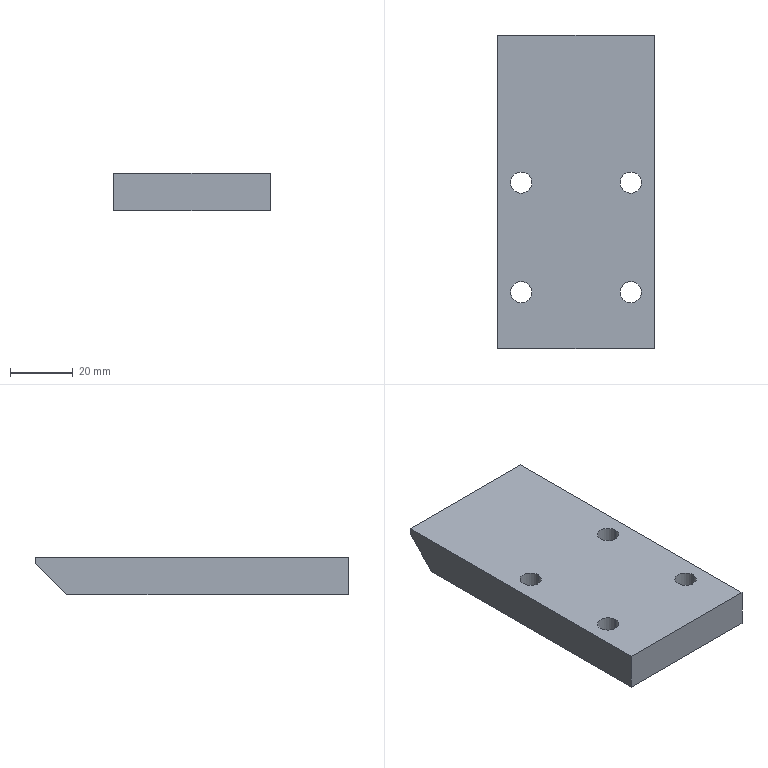Part | STEP file | BCC3 H11_2B1 | 1 solid | 15 faces | box 50 x 100 x 12 mm | volume 55757 mm3 | cylinder 8 | plane 7 | commonest cylinder face diameters 6.8 x8
STEP:
#1=CARTESIAN_POINT('',(0.,0.,0.));
#2=DIRECTION('',(0.,0.,1.));
#3=DIRECTION('',(1.,0.,0.));
#4=AXIS2_PLACEMENT_3D('',#1,#2,#3);
#5=CARTESIAN_POINT('',(-14.1,3.,0.));
#6=VERTEX_POINT('',#5);
#7=CARTESIAN_POINT('',(-14.1,3.,12.));
#8=VERTEX_POINT('',#7);
#9=CARTESIAN_POINT('',(-14.1,3.,12.));
#10=DIRECTION('',(0.,0.,1.));
#11=VECTOR('',#10,1.);
#12=LINE('',#9,#11);
#13=CARTESIAN_POINT('',(-17.5,3.,12.));
#14=DIRECTION('',(0.,0.,1.));
#15=DIRECTION('',(1.,0.,0.));
#16=AXIS2_PLACEMENT_3D('',#13,#14,#15);
#17=CYLINDRICAL_SURFACE('',#16,3.4);
#18=CARTESIAN_POINT('',(6.283,0.));
#19=DIRECTION('',(0.,1.));
#20=VECTOR('',#19,1.);
#21=LINE('',#18,#20);
#22=(GEOMETRIC_REPRESENTATION_CONTEXT(2)PARAMETRIC_REPRESENTATION_CONTEXT()REPRESENTATION_CONTEXT('',''));
#23=DEFINITIONAL_REPRESENTATION('',(#21),#22);
#24=PCURVE('',#17,#23);
#25=CARTESIAN_POINT('',(-17.5,3.,12.));
#26=DIRECTION('',(0.,0.,1.));
#27=DIRECTION('',(1.,0.,0.));
#28=AXIS2_PLACEMENT_3D('',#25,#26,#27);
#29=CYLINDRICAL_SURFACE('',#28,3.4);
#30=CARTESIAN_POINT('',(0.,0.));
#31=DIRECTION('',(0.,1.));
#32=VECTOR('',#31,1.);
#33=LINE('',#30,#32);
#34=(GEOMETRIC_REPRESENTATION_CONTEXT(2)PARAMETRIC_REPRESENTATION_CONTEXT()REPRESENTATION_CONTEXT('',''));
#35=DEFINITIONAL_REPRESENTATION('',(#33),#34);
#36=PCURVE('',#29,#35);
#37=SURFACE_CURVE('',#12,(#24,#36),.PCURVE_S1.);
#38=EDGE_CURVE('',#6,#8,#37,.T.);
#39=ORIENTED_EDGE('',*,*,#38,.T.);
#40=CARTESIAN_POINT('',(-20.9,3.,12.));
#41=VERTEX_POINT('',#40);
#42=CARTESIAN_POINT('',(-17.5,3.,12.));
#43=DIRECTION('',(0.,0.,1.));
#44=DIRECTION('',(1.,0.,0.));
#45=AXIS2_PLACEMENT_3D('',#42,#43,#44);
#46=CIRCLE('',#45,3.4);
#47=CARTESIAN_POINT('',(0.,0.));
#48=DIRECTION('',(1.,0.));
#49=VECTOR('',#48,1.);
#50=LINE('',#47,#49);
#51=(GEOMETRIC_REPRESENTATION_CONTEXT(2)PARAMETRIC_REPRESENTATION_CONTEXT()REPRESENTATION_CONTEXT('',''));
#52=DEFINITIONAL_REPRESENTATION('',(#50),#51);
#53=PCURVE('',#17,#52);
#54=CARTESIAN_POINT('',(0.,0.,12.));
#55=DIRECTION('',(0.,0.,1.));
#56=DIRECTION('',(1.,0.,0.));
#57=AXIS2_PLACEMENT_3D('',#54,#55,#56);
#58=PLANE('',#57);
#59=CARTESIAN_POINT('',(-17.5,3.));
#60=DIRECTION('',(1.,0.));
#61=AXIS2_PLACEMENT_2D('',#59,#60);
#62=CIRCLE('',#61,3.4);
#63=(GEOMETRIC_REPRESENTATION_CONTEXT(2)PARAMETRIC_REPRESENTATION_CONTEXT()REPRESENTATION_CONTEXT('',''));
#64=DEFINITIONAL_REPRESENTATION('',(#62),#63);
#65=PCURVE('',#58,#64);
#66=SURFACE_CURVE('',#46,(#53,#65),.PCURVE_S1.);
#67=EDGE_CURVE('',#41,#8,#66,.T.);
#68=ORIENTED_EDGE('',*,*,#67,.F.);
#69=CARTESIAN_POINT('',(-20.9,3.,0.));
#70=VERTEX_POINT('',#69);
#71=CARTESIAN_POINT('',(-20.9,3.,12.));
#72=DIRECTION('',(0.,0.,1.));
#73=VECTOR('',#72,1.);
#74=LINE('',#71,#73);
#75=CARTESIAN_POINT('',(3.142,0.));
#76=DIRECTION('',(0.,1.));
#77=VECTOR('',#76,1.);
#78=LINE('',#75,#77);
#79=(GEOMETRIC_REPRESENTATION_CONTEXT(2)PARAMETRIC_REPRESENTATION_CONTEXT()REPRESENTATION_CONTEXT('',''));
#80=DEFINITIONAL_REPRESENTATION('',(#78),#79);
#81=PCURVE('',#17,#80);
#82=CARTESIAN_POINT('',(3.142,0.));
#83=DIRECTION('',(0.,1.));
#84=VECTOR('',#83,1.);
#85=LINE('',#82,#84);
#86=(GEOMETRIC_REPRESENTATION_CONTEXT(2)PARAMETRIC_REPRESENTATION_CONTEXT()REPRESENTATION_CONTEXT('',''));
#87=DEFINITIONAL_REPRESENTATION('',(#85),#86);
#88=PCURVE('',#29,#87);
#89=SURFACE_CURVE('',#74,(#81,#88),.PCURVE_S1.);
#90=EDGE_CURVE('',#70,#41,#89,.T.);
#91=ORIENTED_EDGE('',*,*,#90,.F.);
#92=CARTESIAN_POINT('',(-17.5,3.,0.));
#93=DIRECTION('',(0.,0.,1.));
#94=DIRECTION('',(1.,0.,0.));
#95=AXIS2_PLACEMENT_3D('',#92,#93,#94);
#96=CIRCLE('',#95,3.4);
#97=CARTESIAN_POINT('',(0.,-12.));
#98=DIRECTION('',(1.,0.));
#99=VECTOR('',#98,1.);
#100=LINE('',#97,#99);
#101=(GEOMETRIC_REPRESENTATION_CONTEXT(2)PARAMETRIC_REPRESENTATION_CONTEXT()REPRESENTATION_CONTEXT('',''));
#102=DEFINITIONAL_REPRESENTATION('',(#100),#101);
#103=PCURVE('',#17,#102);
#104=CARTESIAN_POINT('',(0.,0.,0.));
#105=DIRECTION('',(0.,0.,1.));
#106=DIRECTION('',(1.,0.,0.));
#107=AXIS2_PLACEMENT_3D('',#104,#105,#106);
#108=PLANE('',#107);
#109=CARTESIAN_POINT('',(-17.5,3.));
#110=DIRECTION('',(1.,0.));
#111=AXIS2_PLACEMENT_2D('',#109,#110);
#112=CIRCLE('',#111,3.4);
#113=(GEOMETRIC_REPRESENTATION_CONTEXT(2)PARAMETRIC_REPRESENTATION_CONTEXT()REPRESENTATION_CONTEXT('',''));
#114=DEFINITIONAL_REPRESENTATION('',(#112),#113);
#115=PCURVE('',#108,#114);
#116=SURFACE_CURVE('',#96,(#103,#115),.PCURVE_S1.);
#117=EDGE_CURVE('',#70,#6,#116,.T.);
#118=ORIENTED_EDGE('',*,*,#117,.T.);
#119=EDGE_LOOP('',(#39,#68,#91,#118));
#120=FACE_BOUND('',#119,.F.);
#121=ADVANCED_FACE('',(#120),#17,.F.);
#122=CARTESIAN_POINT('',(20.9,3.,0.));
#123=VERTEX_POINT('',#122);
#124=CARTESIAN_POINT('',(20.9,3.,12.));
#125=VERTEX_POINT('',#124);
#126=CARTESIAN_POINT('',(20.9,3.,12.));
#127=DIRECTION('',(0.,0.,1.));
#128=VECTOR('',#127,1.);
#129=LINE('',#126,#128);
#130=CARTESIAN_POINT('',(17.5,3.,12.));
#131=DIRECTION('',(0.,0.,1.));
#132=DIRECTION('',(1.,0.,0.));
#133=AXIS2_PLACEMENT_3D('',#130,#131,#132);
#134=CYLINDRICAL_SURFACE('',#133,3.4);
#135=CARTESIAN_POINT('',(6.283,0.));
#136=DIRECTION('',(0.,1.));
#137=VECTOR('',#136,1.);
#138=LINE('',#135,#137);
#139=(GEOMETRIC_REPRESENTATION_CONTEXT(2)PARAMETRIC_REPRESENTATION_CONTEXT()REPRESENTATION_CONTEXT('',''));
#140=DEFINITIONAL_REPRESENTATION('',(#138),#139);
#141=PCURVE('',#134,#140);
#142=CARTESIAN_POINT('',(17.5,3.,12.));
#143=DIRECTION('',(0.,0.,1.));
#144=DIRECTION('',(1.,0.,0.));
#145=AXIS2_PLACEMENT_3D('',#142,#143,#144);
#146=CYLINDRICAL_SURFACE('',#145,3.4);
#147=CARTESIAN_POINT('',(0.,0.));
#148=DIRECTION('',(0.,1.));
#149=VECTOR('',#148,1.);
#150=LINE('',#147,#149);
#151=(GEOMETRIC_REPRESENTATION_CONTEXT(2)PARAMETRIC_REPRESENTATION_CONTEXT()REPRESENTATION_CONTEXT('',''));
#152=DEFINITIONAL_REPRESENTATION('',(#150),#151);
#153=PCURVE('',#146,#152);
#154=SURFACE_CURVE('',#129,(#141,#153),.PCURVE_S1.);
#155=EDGE_CURVE('',#123,#125,#154,.T.);
#156=ORIENTED_EDGE('',*,*,#155,.T.);
#157=CARTESIAN_POINT('',(14.1,3.,12.));
#158=VERTEX_POINT('',#157);
#159=CARTESIAN_POINT('',(17.5,3.,12.));
#160=DIRECTION('',(0.,0.,1.));
#161=DIRECTION('',(1.,0.,0.));
#162=AXIS2_PLACEMENT_3D('',#159,#160,#161);
#163=CIRCLE('',#162,3.4);
#164=CARTESIAN_POINT('',(0.,0.));
#165=DIRECTION('',(1.,0.));
#166=VECTOR('',#165,1.);
#167=LINE('',#164,#166);
#168=(GEOMETRIC_REPRESENTATION_CONTEXT(2)PARAMETRIC_REPRESENTATION_CONTEXT()REPRESENTATION_CONTEXT('',''));
#169=DEFINITIONAL_REPRESENTATION('',(#167),#168);
#170=PCURVE('',#134,#169);
#171=CARTESIAN_POINT('',(17.5,3.));
#172=DIRECTION('',(1.,0.));
#173=AXIS2_PLACEMENT_2D('',#171,#172);
#174=CIRCLE('',#173,3.4);
#175=(GEOMETRIC_REPRESENTATION_CONTEXT(2)PARAMETRIC_REPRESENTATION_CONTEXT()REPRESENTATION_CONTEXT('',''));
#176=DEFINITIONAL_REPRESENTATION('',(#174),#175);
#177=PCURVE('',#58,#176);
#178=SURFACE_CURVE('',#163,(#170,#177),.PCURVE_S1.);
#179=EDGE_CURVE('',#158,#125,#178,.T.);
#180=ORIENTED_EDGE('',*,*,#179,.F.);
#181=CARTESIAN_POINT('',(14.1,3.,0.));
#182=VERTEX_POINT('',#181);
#183=CARTESIAN_POINT('',(14.1,3.,12.));
#184=DIRECTION('',(0.,0.,1.));
#185=VECTOR('',#184,1.);
#186=LINE('',#183,#185);
#187=CARTESIAN_POINT('',(3.142,0.));
#188=DIRECTION('',(0.,1.));
#189=VECTOR('',#188,1.);
#190=LINE('',#187,#189);
#191=(GEOMETRIC_REPRESENTATION_CONTEXT(2)PARAMETRIC_REPRESENTATION_CONTEXT()REPRESENTATION_CONTEXT('',''));
#192=DEFINITIONAL_REPRESENTATION('',(#190),#191);
#193=PCURVE('',#134,#192);
#194=CARTESIAN_POINT('',(3.142,0.));
#195=DIRECTION('',(0.,1.));
#196=VECTOR('',#195,1.);
#197=LINE('',#194,#196);
#198=(GEOMETRIC_REPRESENTATION_CONTEXT(2)PARAMETRIC_REPRESENTATION_CONTEXT()REPRESENTATION_CONTEXT('',''));
#199=DEFINITIONAL_REPRESENTATION('',(#197),#198);
#200=PCURVE('',#146,#199);
#201=SURFACE_CURVE('',#186,(#193,#200),.PCURVE_S1.);
#202=EDGE_CURVE('',#182,#158,#201,.T.);
#203=ORIENTED_EDGE('',*,*,#202,.F.);
#204=CARTESIAN_POINT('',(17.5,3.,0.));
#205=DIRECTION('',(0.,0.,1.));
#206=DIRECTION('',(1.,0.,0.));
#207=AXIS2_PLACEMENT_3D('',#204,#205,#206);
#208=CIRCLE('',#207,3.4);
#209=CARTESIAN_POINT('',(0.,-12.));
#210=DIRECTION('',(1.,0.));
#211=VECTOR('',#210,1.);
#212=LINE('',#209,#211);
#213=(GEOMETRIC_REPRESENTATION_CONTEXT(2)PARAMETRIC_REPRESENTATION_CONTEXT()REPRESENTATION_CONTEXT('',''));
#214=DEFINITIONAL_REPRESENTATION('',(#212),#213);
#215=PCURVE('',#134,#214);
#216=CARTESIAN_POINT('',(17.5,3.));
#217=DIRECTION('',(1.,0.));
#218=AXIS2_PLACEMENT_2D('',#216,#217);
#219=CIRCLE('',#218,3.4);
#220=(GEOMETRIC_REPRESENTATION_CONTEXT(2)PARAMETRIC_REPRESENTATION_CONTEXT()REPRESENTATION_CONTEXT('',''));
#221=DEFINITIONAL_REPRESENTATION('',(#219),#220);
#222=PCURVE('',#108,#221);
#223=SURFACE_CURVE('',#208,(#215,#222),.PCURVE_S1.);
#224=EDGE_CURVE('',#182,#123,#223,.T.);
#225=ORIENTED_EDGE('',*,*,#224,.T.);
#226=EDGE_LOOP('',(#156,#180,#203,#225));
#227=FACE_BOUND('',#226,.F.);
#228=ADVANCED_FACE('',(#227),#134,.F.);
#229=CARTESIAN_POINT('',(20.9,-32.,0.));
#230=VERTEX_POINT('',#229);
#231=CARTESIAN_POINT('',(20.9,-32.,12.));
#232=VERTEX_POINT('',#231);
#233=CARTESIAN_POINT('',(20.9,-32.,12.));
#234=DIRECTION('',(0.,0.,1.));
#235=VECTOR('',#234,1.);
#236=LINE('',#233,#235);
#237=CARTESIAN_POINT('',(17.5,-32.,12.));
#238=DIRECTION('',(0.,0.,1.));
#239=DIRECTION('',(1.,0.,0.));
#240=AXIS2_PLACEMENT_3D('',#237,#238,#239);
#241=CYLINDRICAL_SURFACE('',#240,3.4);
#242=CARTESIAN_POINT('',(6.283,0.));
#243=DIRECTION('',(0.,1.));
#244=VECTOR('',#243,1.);
#245=LINE('',#242,#244);
#246=(GEOMETRIC_REPRESENTATION_CONTEXT(2)PARAMETRIC_REPRESENTATION_CONTEXT()REPRESENTATION_CONTEXT('',''));
#247=DEFINITIONAL_REPRESENTATION('',(#245),#246);
#248=PCURVE('',#241,#247);
#249=CARTESIAN_POINT('',(17.5,-32.,12.));
#250=DIRECTION('',(0.,0.,1.));
#251=DIRECTION('',(1.,0.,0.));
#252=AXIS2_PLACEMENT_3D('',#249,#250,#251);
#253=CYLINDRICAL_SURFACE('',#252,3.4);
#254=CARTESIAN_POINT('',(0.,0.));
#255=DIRECTION('',(0.,1.));
#256=VECTOR('',#255,1.);
#257=LINE('',#254,#256);
#258=(GEOMETRIC_REPRESENTATION_CONTEXT(2)PARAMETRIC_REPRESENTATION_CONTEXT()REPRESENTATION_CONTEXT('',''));
#259=DEFINITIONAL_REPRESENTATION('',(#257),#258);
#260=PCURVE('',#253,#259);
#261=SURFACE_CURVE('',#236,(#248,#260),.PCURVE_S1.);
#262=EDGE_CURVE('',#230,#232,#261,.T.);
#263=ORIENTED_EDGE('',*,*,#262,.T.);
#264=CARTESIAN_POINT('',(14.1,-32.,12.));
#265=VERTEX_POINT('',#264);
#266=CARTESIAN_POINT('',(17.5,-32.,12.));
#267=DIRECTION('',(0.,0.,1.));
#268=DIRECTION('',(1.,0.,0.));
#269=AXIS2_PLACEMENT_3D('',#266,#267,#268);
#270=CIRCLE('',#269,3.4);
#271=CARTESIAN_POINT('',(0.,0.));
#272=DIRECTION('',(1.,0.));
#273=VECTOR('',#272,1.);
#274=LINE('',#271,#273);
#275=(GEOMETRIC_REPRESENTATION_CONTEXT(2)PARAMETRIC_REPRESENTATION_CONTEXT()REPRESENTATION_CONTEXT('',''));
#276=DEFINITIONAL_REPRESENTATION('',(#274),#275);
#277=PCURVE('',#241,#276);
#278=CARTESIAN_POINT('',(17.5,-32.));
#279=DIRECTION('',(1.,0.));
#280=AXIS2_PLACEMENT_2D('',#278,#279);
#281=CIRCLE('',#280,3.4);
#282=(GEOMETRIC_REPRESENTATION_CONTEXT(2)PARAMETRIC_REPRESENTATION_CONTEXT()REPRESENTATION_CONTEXT('',''));
#283=DEFINITIONAL_REPRESENTATION('',(#281),#282);
#284=PCURVE('',#58,#283);
#285=SURFACE_CURVE('',#270,(#277,#284),.PCURVE_S1.);
#286=EDGE_CURVE('',#265,#232,#285,.T.);
#287=ORIENTED_EDGE('',*,*,#286,.F.);
#288=CARTESIAN_POINT('',(14.1,-32.,0.));
#289=VERTEX_POINT('',#288);
#290=CARTESIAN_POINT('',(14.1,-32.,12.));
#291=DIRECTION('',(0.,0.,1.));
#292=VECTOR('',#291,1.);
#293=LINE('',#290,#292);
#294=CARTESIAN_POINT('',(3.142,0.));
#295=DIRECTION('',(0.,1.));
#296=VECTOR('',#295,1.);
#297=LINE('',#294,#296);
#298=(GEOMETRIC_REPRESENTATION_CONTEXT(2)PARAMETRIC_REPRESENTATION_CONTEXT()REPRESENTATION_CONTEXT('',''));
#299=DEFINITIONAL_REPRESENTATION('',(#297),#298);
#300=PCURVE('',#241,#299);
#301=CARTESIAN_POINT('',(3.142,0.));
#302=DIRECTION('',(0.,1.));
#303=VECTOR('',#302,1.);
#304=LINE('',#301,#303);
#305=(GEOMETRIC_REPRESENTATION_CONTEXT(2)PARAMETRIC_REPRESENTATION_CONTEXT()REPRESENTATION_CONTEXT('',''));
#306=DEFINITIONAL_REPRESENTATION('',(#304),#305);
#307=PCURVE('',#253,#306);
#308=SURFACE_CURVE('',#293,(#300,#307),.PCURVE_S1.);
#309=EDGE_CURVE('',#289,#265,#308,.T.);
#310=ORIENTED_EDGE('',*,*,#309,.F.);
#311=CARTESIAN_POINT('',(17.5,-32.,0.));
#312=DIRECTION('',(0.,0.,1.));
#313=DIRECTION('',(1.,0.,0.));
#314=AXIS2_PLACEMENT_3D('',#311,#312,#313);
#315=CIRCLE('',#314,3.4);
#316=CARTESIAN_POINT('',(0.,-12.));
#317=DIRECTION('',(1.,0.));
#318=VECTOR('',#317,1.);
#319=LINE('',#316,#318);
#320=(GEOMETRIC_REPRESENTATION_CONTEXT(2)PARAMETRIC_REPRESENTATION_CONTEXT()REPRESENTATION_CONTEXT('',''));
#321=DEFINITIONAL_REPRESENTATION('',(#319),#320);
#322=PCURVE('',#241,#321);
#323=CARTESIAN_POINT('',(17.5,-32.));
#324=DIRECTION('',(1.,0.));
#325=AXIS2_PLACEMENT_2D('',#323,#324);
#326=CIRCLE('',#325,3.4);
#327=(GEOMETRIC_REPRESENTATION_CONTEXT(2)PARAMETRIC_REPRESENTATION_CONTEXT()REPRESENTATION_CONTEXT('',''));
#328=DEFINITIONAL_REPRESENTATION('',(#326),#327);
#329=PCURVE('',#108,#328);
#330=SURFACE_CURVE('',#315,(#322,#329),.PCURVE_S1.);
#331=EDGE_CURVE('',#289,#230,#330,.T.);
#332=ORIENTED_EDGE('',*,*,#331,.T.);
#333=EDGE_LOOP('',(#263,#287,#310,#332));
#334=FACE_BOUND('',#333,.F.);
#335=ADVANCED_FACE('',(#334),#241,.F.);
#336=CARTESIAN_POINT('',(-14.1,-32.,0.));
#337=VERTEX_POINT('',#336);
#338=CARTESIAN_POINT('',(-14.1,-32.,12.));
#339=VERTEX_POINT('',#338);
#340=CARTESIAN_POINT('',(-14.1,-32.,12.));
#341=DIRECTION('',(0.,0.,1.));
#342=VECTOR('',#341,1.);
#343=LINE('',#340,#342);
#344=CARTESIAN_POINT('',(-17.5,-32.,12.));
#345=DIRECTION('',(0.,0.,1.));
#346=DIRECTION('',(1.,0.,0.));
#347=AXIS2_PLACEMENT_3D('',#344,#345,#346);
#348=CYLINDRICAL_SURFACE('',#347,3.4);
#349=CARTESIAN_POINT('',(6.283,0.));
#350=DIRECTION('',(0.,1.));
#351=VECTOR('',#350,1.);
#352=LINE('',#349,#351);
#353=(GEOMETRIC_REPRESENTATION_CONTEXT(2)PARAMETRIC_REPRESENTATION_CONTEXT()REPRESENTATION_CONTEXT('',''));
#354=DEFINITIONAL_REPRESENTATION('',(#352),#353);
#355=PCURVE('',#348,#354);
#356=CARTESIAN_POINT('',(-17.5,-32.,12.));
#357=DIRECTION('',(0.,0.,1.));
#358=DIRECTION('',(1.,0.,0.));
#359=AXIS2_PLACEMENT_3D('',#356,#357,#358);
#360=CYLINDRICAL_SURFACE('',#359,3.4);
#361=CARTESIAN_POINT('',(0.,0.));
#362=DIRECTION('',(0.,1.));
#363=VECTOR('',#362,1.);
#364=LINE('',#361,#363);
#365=(GEOMETRIC_REPRESENTATION_CONTEXT(2)PARAMETRIC_REPRESENTATION_CONTEXT()REPRESENTATION_CONTEXT('',''));
#366=DEFINITIONAL_REPRESENTATION('',(#364),#365);
#367=PCURVE('',#360,#366);
#368=SURFACE_CURVE('',#343,(#355,#367),.PCURVE_S1.);
#369=EDGE_CURVE('',#337,#339,#368,.T.);
#370=ORIENTED_EDGE('',*,*,#369,.T.);
#371=CARTESIAN_POINT('',(-20.9,-32.,12.));
#372=VERTEX_POINT('',#371);
#373=CARTESIAN_POINT('',(-17.5,-32.,12.));
#374=DIRECTION('',(0.,0.,1.));
#375=DIRECTION('',(1.,0.,0.));
#376=AXIS2_PLACEMENT_3D('',#373,#374,#375);
#377=CIRCLE('',#376,3.4);
#378=CARTESIAN_POINT('',(0.,0.));
#379=DIRECTION('',(1.,0.));
#380=VECTOR('',#379,1.);
#381=LINE('',#378,#380);
#382=(GEOMETRIC_REPRESENTATION_CONTEXT(2)PARAMETRIC_REPRESENTATION_CONTEXT()REPRESENTATION_CONTEXT('',''));
#383=DEFINITIONAL_REPRESENTATION('',(#381),#382);
#384=PCURVE('',#348,#383);
#385=CARTESIAN_POINT('',(-17.5,-32.));
#386=DIRECTION('',(1.,0.));
#387=AXIS2_PLACEMENT_2D('',#385,#386);
#388=CIRCLE('',#387,3.4);
#389=(GEOMETRIC_REPRESENTATION_CONTEXT(2)PARAMETRIC_REPRESENTATION_CONTEXT()REPRESENTATION_CONTEXT('',''));
#390=DEFINITIONAL_REPRESENTATION('',(#388),#389);
#391=PCURVE('',#58,#390);
#392=SURFACE_CURVE('',#377,(#384,#391),.PCURVE_S1.);
#393=EDGE_CURVE('',#372,#339,#392,.T.);
#394=ORIENTED_EDGE('',*,*,#393,.F.);
#395=CARTESIAN_POINT('',(-20.9,-32.,0.));
#396=VERTEX_POINT('',#395);
#397=CARTESIAN_POINT('',(-20.9,-32.,12.));
#398=DIRECTION('',(0.,0.,1.));
#399=VECTOR('',#398,1.);
#400=LINE('',#397,#399);
#401=CARTESIAN_POINT('',(3.142,0.));
#402=DIRECTION('',(0.,1.));
#403=VECTOR('',#402,1.);
#404=LINE('',#401,#403);
#405=(GEOMETRIC_REPRESENTATION_CONTEXT(2)PARAMETRIC_REPRESENTATION_CONTEXT()REPRESENTATION_CONTEXT('',''));
#406=DEFINITIONAL_REPRESENTATION('',(#404),#405);
#407=PCURVE('',#348,#406);
#408=CARTESIAN_POINT('',(3.142,0.));
#409=DIRECTION('',(0.,1.));
#410=VECTOR('',#409,1.);
#411=LINE('',#408,#410);
#412=(GEOMETRIC_REPRESENTATION_CONTEXT(2)PARAMETRIC_REPRESENTATION_CONTEXT()REPRESENTATION_CONTEXT('',''));
#413=DEFINITIONAL_REPRESENTATION('',(#411),#412);
#414=PCURVE('',#360,#413);
#415=SURFACE_CURVE('',#400,(#407,#414),.PCURVE_S1.);
#416=EDGE_CURVE('',#396,#372,#415,.T.);
#417=ORIENTED_EDGE('',*,*,#416,.F.);
#418=CARTESIAN_POINT('',(-17.5,-32.,0.));
#419=DIRECTION('',(0.,0.,1.));
#420=DIRECTION('',(1.,0.,0.));
#421=AXIS2_PLACEMENT_3D('',#418,#419,#420);
#422=CIRCLE('',#421,3.4);
#423=CARTESIAN_POINT('',(0.,-12.));
#424=DIRECTION('',(1.,0.));
#425=VECTOR('',#424,1.);
#426=LINE('',#423,#425);
#427=(GEOMETRIC_REPRESENTATION_CONTEXT(2)PARAMETRIC_REPRESENTATION_CONTEXT()REPRESENTATION_CONTEXT('',''));
#428=DEFINITIONAL_REPRESENTATION('',(#426),#427);
#429=PCURVE('',#348,#428);
#430=CARTESIAN_POINT('',(-17.5,-32.));
#431=DIRECTION('',(1.,0.));
#432=AXIS2_PLACEMENT_2D('',#430,#431);
#433=CIRCLE('',#432,3.4);
#434=(GEOMETRIC_REPRESENTATION_CONTEXT(2)PARAMETRIC_REPRESENTATION_CONTEXT()REPRESENTATION_CONTEXT('',''));
#435=DEFINITIONAL_REPRESENTATION('',(#433),#434);
#436=PCURVE('',#108,#435);
#437=SURFACE_CURVE('',#422,(#429,#436),.PCURVE_S1.);
#438=EDGE_CURVE('',#396,#337,#437,.T.);
#439=ORIENTED_EDGE('',*,*,#438,.T.);
#440=EDGE_LOOP('',(#370,#394,#417,#439));
#441=FACE_BOUND('',#440,.F.);
#442=ADVANCED_FACE('',(#441),#348,.F.);
#443=CARTESIAN_POINT('',(-25.,50.,12.));
#444=VERTEX_POINT('',#443);
#445=CARTESIAN_POINT('',(-25.,50.,10.));
#446=VERTEX_POINT('',#445);
#447=CARTESIAN_POINT('',(-25.,50.,12.));
#448=DIRECTION('',(0.,0.,-1.));
#449=VECTOR('',#448,1.);
#450=LINE('',#447,#449);
#451=CARTESIAN_POINT('',(-25.,50.,12.));
#452=DIRECTION('',(1.,0.,0.));
#453=DIRECTION('',(0.,1.,0.));
#454=AXIS2_PLACEMENT_3D('',#451,#452,#453);
#455=PLANE('',#454);
#456=CARTESIAN_POINT('',(0.,0.));
#457=DIRECTION('',(0.,-1.));
#458=VECTOR('',#457,1.);
#459=LINE('',#456,#458);
#460=(GEOMETRIC_REPRESENTATION_CONTEXT(2)PARAMETRIC_REPRESENTATION_CONTEXT()REPRESENTATION_CONTEXT('',''));
#461=DEFINITIONAL_REPRESENTATION('',(#459),#460);
#462=PCURVE('',#455,#461);
#463=CARTESIAN_POINT('',(-25.,50.,12.));
#464=DIRECTION('',(0.,-1.,0.));
#465=DIRECTION('',(0.,0.,-1.));
#466=AXIS2_PLACEMENT_3D('',#463,#464,#465);
#467=PLANE('',#466);
#468=CARTESIAN_POINT('',(0.,0.));
#469=DIRECTION('',(1.,0.));
#470=VECTOR('',#469,1.);
#471=LINE('',#468,#470);
#472=(GEOMETRIC_REPRESENTATION_CONTEXT(2)PARAMETRIC_REPRESENTATION_CONTEXT()REPRESENTATION_CONTEXT('',''));
#473=DEFINITIONAL_REPRESENTATION('',(#471),#472);
#474=PCURVE('',#467,#473);
#475=SURFACE_CURVE('',#450,(#462,#474),.PCURVE_S1.);
#476=EDGE_CURVE('',#444,#446,#475,.T.);
#477=ORIENTED_EDGE('',*,*,#476,.T.);
#478=CARTESIAN_POINT('',(-25.,40.,0.));
#479=VERTEX_POINT('',#478);
#480=CARTESIAN_POINT('',(-25.,50.,10.));
#481=DIRECTION('',(0.,-0.7071,-0.7071));
#482=VECTOR('',#481,1.);
#483=LINE('',#480,#482);
#484=CARTESIAN_POINT('',(0.,-2.));
#485=DIRECTION('',(-0.7071,-0.7071));
#486=VECTOR('',#485,1.);
#487=LINE('',#484,#486);
#488=(GEOMETRIC_REPRESENTATION_CONTEXT(2)PARAMETRIC_REPRESENTATION_CONTEXT()REPRESENTATION_CONTEXT('',''));
#489=DEFINITIONAL_REPRESENTATION('',(#487),#488);
#490=PCURVE('',#455,#489);
#491=CARTESIAN_POINT('',(-25.,50.,10.));
#492=DIRECTION('',(0.,-0.7071,0.7071));
#493=DIRECTION('',(-1.,0.,0.));
#494=AXIS2_PLACEMENT_3D('',#491,#492,#493);
#495=PLANE('',#494);
#496=CARTESIAN_POINT('',(0.,0.));
#497=DIRECTION('',(0.,1.));
#498=VECTOR('',#497,1.);
#499=LINE('',#496,#498);
#500=(GEOMETRIC_REPRESENTATION_CONTEXT(2)PARAMETRIC_REPRESENTATION_CONTEXT()REPRESENTATION_CONTEXT('',''));
#501=DEFINITIONAL_REPRESENTATION('',(#499),#500);
#502=PCURVE('',#495,#501);
#503=SURFACE_CURVE('',#483,(#490,#502),.PCURVE_S1.);
#504=EDGE_CURVE('',#446,#479,#503,.T.);
#505=ORIENTED_EDGE('',*,*,#504,.T.);
#506=CARTESIAN_POINT('',(-25.,-50.,0.));
#507=VERTEX_POINT('',#506);
#508=CARTESIAN_POINT('',(-25.,50.,0.));
#509=DIRECTION('',(0.,-1.,0.));
#510=VECTOR('',#509,1.);
#511=LINE('',#508,#510);
#512=CARTESIAN_POINT('',(0.,-12.));
#513=DIRECTION('',(-1.,0.));
#514=VECTOR('',#513,1.);
#515=LINE('',#512,#514);
#516=(GEOMETRIC_REPRESENTATION_CONTEXT(2)PARAMETRIC_REPRESENTATION_CONTEXT()REPRESENTATION_CONTEXT('',''));
#517=DEFINITIONAL_REPRESENTATION('',(#515),#516);
#518=PCURVE('',#455,#517);
#519=CARTESIAN_POINT('',(-25.,50.));
#520=DIRECTION('',(0.,-1.));
#521=VECTOR('',#520,1.);
#522=LINE('',#519,#521);
#523=(GEOMETRIC_REPRESENTATION_CONTEXT(2)PARAMETRIC_REPRESENTATION_CONTEXT()REPRESENTATION_CONTEXT('',''));
#524=DEFINITIONAL_REPRESENTATION('',(#522),#523);
#525=PCURVE('',#108,#524);
#526=SURFACE_CURVE('',#511,(#518,#525),.PCURVE_S1.);
#527=EDGE_CURVE('',#479,#507,#526,.T.);
#528=ORIENTED_EDGE('',*,*,#527,.T.);
#529=CARTESIAN_POINT('',(-25.,-50.,12.));
#530=VERTEX_POINT('',#529);
#531=CARTESIAN_POINT('',(-25.,-50.,12.));
#532=DIRECTION('',(0.,0.,-1.));
#533=VECTOR('',#532,1.);
#534=LINE('',#531,#533);
#535=CARTESIAN_POINT('',(-100.,0.));
#536=DIRECTION('',(0.,-1.));
#537=VECTOR('',#536,1.);
#538=LINE('',#535,#537);
#539=(GEOMETRIC_REPRESENTATION_CONTEXT(2)PARAMETRIC_REPRESENTATION_CONTEXT()REPRESENTATION_CONTEXT('',''));
#540=DEFINITIONAL_REPRESENTATION('',(#538),#539);
#541=PCURVE('',#455,#540);
#542=CARTESIAN_POINT('',(-25.,-50.,12.));
#543=DIRECTION('',(0.,1.,0.));
#544=DIRECTION('',(0.,0.,1.));
#545=AXIS2_PLACEMENT_3D('',#542,#543,#544);
#546=PLANE('',#545);
#547=CARTESIAN_POINT('',(0.,0.));
#548=DIRECTION('',(-1.,0.));
#549=VECTOR('',#548,1.);
#550=LINE('',#547,#549);
#551=(GEOMETRIC_REPRESENTATION_CONTEXT(2)PARAMETRIC_REPRESENTATION_CONTEXT()REPRESENTATION_CONTEXT('',''));
#552=DEFINITIONAL_REPRESENTATION('',(#550),#551);
#553=PCURVE('',#546,#552);
#554=SURFACE_CURVE('',#534,(#541,#553),.PCURVE_S1.);
#555=EDGE_CURVE('',#530,#507,#554,.T.);
#556=ORIENTED_EDGE('',*,*,#555,.F.);
#557=CARTESIAN_POINT('',(-25.,50.,12.));
#558=DIRECTION('',(0.,-1.,0.));
#559=VECTOR('',#558,1.);
#560=LINE('',#557,#559);
#561=CARTESIAN_POINT('',(0.,0.));
#562=DIRECTION('',(-1.,0.));
#563=VECTOR('',#562,1.);
#564=LINE('',#561,#563);
#565=(GEOMETRIC_REPRESENTATION_CONTEXT(2)PARAMETRIC_REPRESENTATION_CONTEXT()REPRESENTATION_CONTEXT('',''));
#566=DEFINITIONAL_REPRESENTATION('',(#564),#565);
#567=PCURVE('',#455,#566);
#568=CARTESIAN_POINT('',(-25.,50.));
#569=DIRECTION('',(0.,-1.));
#570=VECTOR('',#569,1.);
#571=LINE('',#568,#570);
#572=(GEOMETRIC_REPRESENTATION_CONTEXT(2)PARAMETRIC_REPRESENTATION_CONTEXT()REPRESENTATION_CONTEXT('',''));
#573=DEFINITIONAL_REPRESENTATION('',(#571),#572);
#574=PCURVE('',#58,#573);
#575=SURFACE_CURVE('',#560,(#567,#574),.PCURVE_S1.);
#576=EDGE_CURVE('',#444,#530,#575,.T.);
#577=ORIENTED_EDGE('',*,*,#576,.F.);
#578=EDGE_LOOP('',(#477,#505,#528,#556,#577));
#579=FACE_BOUND('',#578,.T.);
#580=ADVANCED_FACE('',(#579),#455,.F.);
#581=CARTESIAN_POINT('',(25.,-50.,0.));
#582=VERTEX_POINT('',#581);
#583=CARTESIAN_POINT('',(-25.,-50.,0.));
#584=DIRECTION('',(1.,0.,0.));
#585=VECTOR('',#584,1.);
#586=LINE('',#583,#585);
#587=CARTESIAN_POINT('',(-12.,0.));
#588=DIRECTION('',(0.,1.));
#589=VECTOR('',#588,1.);
#590=LINE('',#587,#589);
#591=(GEOMETRIC_REPRESENTATION_CONTEXT(2)PARAMETRIC_REPRESENTATION_CONTEXT()REPRESENTATION_CONTEXT('',''));
#592=DEFINITIONAL_REPRESENTATION('',(#590),#591);
#593=PCURVE('',#546,#592);
#594=CARTESIAN_POINT('',(-25.,-50.));
#595=DIRECTION('',(1.,0.));
#596=VECTOR('',#595,1.);
#597=LINE('',#594,#596);
#598=(GEOMETRIC_REPRESENTATION_CONTEXT(2)PARAMETRIC_REPRESENTATION_CONTEXT()REPRESENTATION_CONTEXT('',''));
#599=DEFINITIONAL_REPRESENTATION('',(#597),#598);
#600=PCURVE('',#108,#599);
#601=SURFACE_CURVE('',#586,(#593,#600),.PCURVE_S1.);
#602=EDGE_CURVE('',#507,#582,#601,.T.);
#603=ORIENTED_EDGE('',*,*,#602,.T.);
#604=CARTESIAN_POINT('',(25.,-50.,12.));
#605=VERTEX_POINT('',#604);
#606=CARTESIAN_POINT('',(25.,-50.,12.));
#607=DIRECTION('',(0.,0.,-1.));
#608=VECTOR('',#607,1.);
#609=LINE('',#606,#608);
#610=CARTESIAN_POINT('',(0.,50.));
#611=DIRECTION('',(-1.,0.));
#612=VECTOR('',#611,1.);
#613=LINE('',#610,#612);
#614=(GEOMETRIC_REPRESENTATION_CONTEXT(2)PARAMETRIC_REPRESENTATION_CONTEXT()REPRESENTATION_CONTEXT('',''));
#615=DEFINITIONAL_REPRESENTATION('',(#613),#614);
#616=PCURVE('',#546,#615);
#617=CARTESIAN_POINT('',(25.,50.,12.));
#618=DIRECTION('',(-1.,0.,0.));
#619=DIRECTION('',(0.,-1.,0.));
#620=AXIS2_PLACEMENT_3D('',#617,#618,#619);
#621=PLANE('',#620);
#622=CARTESIAN_POINT('',(100.,0.));
#623=DIRECTION('',(0.,-1.));
#624=VECTOR('',#623,1.);
#625=LINE('',#622,#624);
#626=(GEOMETRIC_REPRESENTATION_CONTEXT(2)PARAMETRIC_REPRESENTATION_CONTEXT()REPRESENTATION_CONTEXT('',''));
#627=DEFINITIONAL_REPRESENTATION('',(#625),#626);
#628=PCURVE('',#621,#627);
#629=SURFACE_CURVE('',#609,(#616,#628),.PCURVE_S1.);
#630=EDGE_CURVE('',#605,#582,#629,.T.);
#631=ORIENTED_EDGE('',*,*,#630,.F.);
#632=CARTESIAN_POINT('',(-25.,-50.,12.));
#633=DIRECTION('',(1.,0.,0.));
#634=VECTOR('',#633,1.);
#635=LINE('',#632,#634);
#636=CARTESIAN_POINT('',(0.,0.));
#637=DIRECTION('',(0.,1.));
#638=VECTOR('',#637,1.);
#639=LINE('',#636,#638);
#640=(GEOMETRIC_REPRESENTATION_CONTEXT(2)PARAMETRIC_REPRESENTATION_CONTEXT()REPRESENTATION_CONTEXT('',''));
#641=DEFINITIONAL_REPRESENTATION('',(#639),#640);
#642=PCURVE('',#546,#641);
#643=CARTESIAN_POINT('',(-25.,-50.));
#644=DIRECTION('',(1.,0.));
#645=VECTOR('',#644,1.);
#646=LINE('',#643,#645);
#647=(GEOMETRIC_REPRESENTATION_CONTEXT(2)PARAMETRIC_REPRESENTATION_CONTEXT()REPRESENTATION_CONTEXT('',''));
#648=DEFINITIONAL_REPRESENTATION('',(#646),#647);
#649=PCURVE('',#58,#648);
#650=SURFACE_CURVE('',#635,(#642,#649),.PCURVE_S1.);
#651=EDGE_CURVE('',#530,#605,#650,.T.);
#652=ORIENTED_EDGE('',*,*,#651,.F.);
#653=ORIENTED_EDGE('',*,*,#555,.T.);
#654=EDGE_LOOP('',(#603,#631,#652,#653));
#655=FACE_BOUND('',#654,.T.);
#656=ADVANCED_FACE('',(#655),#546,.F.);
#657=CARTESIAN_POINT('',(25.,40.,0.));
#658=VERTEX_POINT('',#657);
#659=CARTESIAN_POINT('',(25.,50.,0.));
#660=DIRECTION('',(0.,1.,0.));
#661=VECTOR('',#660,1.);
#662=LINE('',#659,#661);
#663=CARTESIAN_POINT('',(0.,-12.));
#664=DIRECTION('',(-1.,0.));
#665=VECTOR('',#664,1.);
#666=LINE('',#663,#665);
#667=(GEOMETRIC_REPRESENTATION_CONTEXT(2)PARAMETRIC_REPRESENTATION_CONTEXT()REPRESENTATION_CONTEXT('',''));
#668=DEFINITIONAL_REPRESENTATION('',(#666),#667);
#669=PCURVE('',#621,#668);
#670=CARTESIAN_POINT('',(25.,50.));
#671=DIRECTION('',(0.,1.));
#672=VECTOR('',#671,1.);
#673=LINE('',#670,#672);
#674=(GEOMETRIC_REPRESENTATION_CONTEXT(2)PARAMETRIC_REPRESENTATION_CONTEXT()REPRESENTATION_CONTEXT('',''));
#675=DEFINITIONAL_REPRESENTATION('',(#673),#674);
#676=PCURVE('',#108,#675);
#677=SURFACE_CURVE('',#662,(#669,#676),.PCURVE_S1.);
#678=EDGE_CURVE('',#582,#658,#677,.T.);
#679=ORIENTED_EDGE('',*,*,#678,.T.);
#680=CARTESIAN_POINT('',(25.,50.,10.));
#681=VERTEX_POINT('',#680);
#682=CARTESIAN_POINT('',(25.,50.,10.));
#683=DIRECTION('',(0.,0.7071,0.7071));
#684=VECTOR('',#683,1.);
#685=LINE('',#682,#684);
#686=CARTESIAN_POINT('',(0.,-2.));
#687=DIRECTION('',(-0.7071,0.7071));
#688=VECTOR('',#687,1.);
#689=LINE('',#686,#688);
#690=(GEOMETRIC_REPRESENTATION_CONTEXT(2)PARAMETRIC_REPRESENTATION_CONTEXT()REPRESENTATION_CONTEXT('',''));
#691=DEFINITIONAL_REPRESENTATION('',(#689),#690);
#692=PCURVE('',#621,#691);
#693=CARTESIAN_POINT('',(-50.,0.));
#694=DIRECTION('',(0.,-1.));
#695=VECTOR('',#694,1.);
#696=LINE('',#693,#695);
#697=(GEOMETRIC_REPRESENTATION_CONTEXT(2)PARAMETRIC_REPRESENTATION_CONTEXT()REPRESENTATION_CONTEXT('',''));
#698=DEFINITIONAL_REPRESENTATION('',(#696),#697);
#699=PCURVE('',#495,#698);
#700=SURFACE_CURVE('',#685,(#692,#699),.PCURVE_S1.);
#701=EDGE_CURVE('',#658,#681,#700,.T.);
#702=ORIENTED_EDGE('',*,*,#701,.T.);
#703=CARTESIAN_POINT('',(25.,50.,12.));
#704=VERTEX_POINT('',#703);
#705=CARTESIAN_POINT('',(25.,50.,12.));
#706=DIRECTION('',(0.,0.,-1.));
#707=VECTOR('',#706,1.);
#708=LINE('',#705,#707);
#709=CARTESIAN_POINT('',(0.,0.));
#710=DIRECTION('',(0.,-1.));
#711=VECTOR('',#710,1.);
#712=LINE('',#709,#711);
#713=(GEOMETRIC_REPRESENTATION_CONTEXT(2)PARAMETRIC_REPRESENTATION_CONTEXT()REPRESENTATION_CONTEXT('',''));
#714=DEFINITIONAL_REPRESENTATION('',(#712),#713);
#715=PCURVE('',#621,#714);
#716=CARTESIAN_POINT('',(0.,50.));
#717=DIRECTION('',(1.,0.));
#718=VECTOR('',#717,1.);
#719=LINE('',#716,#718);
#720=(GEOMETRIC_REPRESENTATION_CONTEXT(2)PARAMETRIC_REPRESENTATION_CONTEXT()REPRESENTATION_CONTEXT('',''));
#721=DEFINITIONAL_REPRESENTATION('',(#719),#720);
#722=PCURVE('',#467,#721);
#723=SURFACE_CURVE('',#708,(#715,#722),.PCURVE_S1.);
#724=EDGE_CURVE('',#704,#681,#723,.T.);
#725=ORIENTED_EDGE('',*,*,#724,.F.);
#726=CARTESIAN_POINT('',(25.,50.,12.));
#727=DIRECTION('',(0.,1.,0.));
#728=VECTOR('',#727,1.);
#729=LINE('',#726,#728);
#730=CARTESIAN_POINT('',(0.,0.));
#731=DIRECTION('',(-1.,0.));
#732=VECTOR('',#731,1.);
#733=LINE('',#730,#732);
#734=(GEOMETRIC_REPRESENTATION_CONTEXT(2)PARAMETRIC_REPRESENTATION_CONTEXT()REPRESENTATION_CONTEXT('',''));
#735=DEFINITIONAL_REPRESENTATION('',(#733),#734);
#736=PCURVE('',#621,#735);
#737=CARTESIAN_POINT('',(25.,50.));
#738=DIRECTION('',(0.,1.));
#739=VECTOR('',#738,1.);
#740=LINE('',#737,#739);
#741=(GEOMETRIC_REPRESENTATION_CONTEXT(2)PARAMETRIC_REPRESENTATION_CONTEXT()REPRESENTATION_CONTEXT('',''));
#742=DEFINITIONAL_REPRESENTATION('',(#740),#741);
#743=PCURVE('',#58,#742);
#744=SURFACE_CURVE('',#729,(#736,#743),.PCURVE_S1.);
#745=EDGE_CURVE('',#605,#704,#744,.T.);
#746=ORIENTED_EDGE('',*,*,#745,.F.);
#747=ORIENTED_EDGE('',*,*,#630,.T.);
#748=EDGE_LOOP('',(#679,#702,#725,#746,#747));
#749=FACE_BOUND('',#748,.T.);
#750=ADVANCED_FACE('',(#749),#621,.F.);
#751=ORIENTED_EDGE('',*,*,#724,.T.);
#752=CARTESIAN_POINT('',(-25.,50.,10.));
#753=DIRECTION('',(-1.,0.,0.));
#754=VECTOR('',#753,1.);
#755=LINE('',#752,#754);
#756=CARTESIAN_POINT('',(2.,0.));
#757=DIRECTION('',(0.,-1.));
#758=VECTOR('',#757,1.);
#759=LINE('',#756,#758);
#760=(GEOMETRIC_REPRESENTATION_CONTEXT(2)PARAMETRIC_REPRESENTATION_CONTEXT()REPRESENTATION_CONTEXT('',''));
#761=DEFINITIONAL_REPRESENTATION('',(#759),#760);
#762=PCURVE('',#467,#761);
#763=CARTESIAN_POINT('',(0.,0.));
#764=DIRECTION('',(1.,0.));
#765=VECTOR('',#764,1.);
#766=LINE('',#763,#765);
#767=(GEOMETRIC_REPRESENTATION_CONTEXT(2)PARAMETRIC_REPRESENTATION_CONTEXT()REPRESENTATION_CONTEXT('',''));
#768=DEFINITIONAL_REPRESENTATION('',(#766),#767);
#769=PCURVE('',#495,#768);
#770=SURFACE_CURVE('',#755,(#762,#769),.PCURVE_S1.);
#771=EDGE_CURVE('',#681,#446,#770,.T.);
#772=ORIENTED_EDGE('',*,*,#771,.T.);
#773=ORIENTED_EDGE('',*,*,#476,.F.);
#774=CARTESIAN_POINT('',(-25.,50.,12.));
#775=DIRECTION('',(-1.,0.,0.));
#776=VECTOR('',#775,1.);
#777=LINE('',#774,#776);
#778=CARTESIAN_POINT('',(0.,0.));
#779=DIRECTION('',(0.,-1.));
#780=VECTOR('',#779,1.);
#781=LINE('',#778,#780);
#782=(GEOMETRIC_REPRESENTATION_CONTEXT(2)PARAMETRIC_REPRESENTATION_CONTEXT()REPRESENTATION_CONTEXT('',''));
#783=DEFINITIONAL_REPRESENTATION('',(#781),#782);
#784=PCURVE('',#467,#783);
#785=CARTESIAN_POINT('',(-25.,50.));
#786=DIRECTION('',(-1.,0.));
#787=VECTOR('',#786,1.);
#788=LINE('',#785,#787);
#789=(GEOMETRIC_REPRESENTATION_CONTEXT(2)PARAMETRIC_REPRESENTATION_CONTEXT()REPRESENTATION_CONTEXT('',''));
#790=DEFINITIONAL_REPRESENTATION('',(#788),#789);
#791=PCURVE('',#58,#790);
#792=SURFACE_CURVE('',#777,(#784,#791),.PCURVE_S1.);
#793=EDGE_CURVE('',#704,#444,#792,.T.);
#794=ORIENTED_EDGE('',*,*,#793,.F.);
#795=EDGE_LOOP('',(#751,#772,#773,#794));
#796=FACE_BOUND('',#795,.T.);
#797=ADVANCED_FACE('',(#796),#467,.F.);
#798=CARTESIAN_POINT('',(-17.5,3.,12.));
#799=DIRECTION('',(0.,0.,1.));
#800=DIRECTION('',(1.,0.,0.));
#801=AXIS2_PLACEMENT_3D('',#798,#799,#800);
#802=CIRCLE('',#801,3.4);
#803=CARTESIAN_POINT('',(-17.5,3.));
#804=DIRECTION('',(1.,0.));
#805=AXIS2_PLACEMENT_2D('',#803,#804);
#806=CIRCLE('',#805,3.4);
#807=(GEOMETRIC_REPRESENTATION_CONTEXT(2)PARAMETRIC_REPRESENTATION_CONTEXT()REPRESENTATION_CONTEXT('',''));
#808=DEFINITIONAL_REPRESENTATION('',(#806),#807);
#809=PCURVE('',#58,#808);
#810=CARTESIAN_POINT('',(0.,0.));
#811=DIRECTION('',(1.,0.));
#812=VECTOR('',#811,1.);
#813=LINE('',#810,#812);
#814=(GEOMETRIC_REPRESENTATION_CONTEXT(2)PARAMETRIC_REPRESENTATION_CONTEXT()REPRESENTATION_CONTEXT('',''));
#815=DEFINITIONAL_REPRESENTATION('',(#813),#814);
#816=PCURVE('',#29,#815);
#817=SURFACE_CURVE('',#802,(#809,#816),.PCURVE_S1.);
#818=EDGE_CURVE('',#8,#41,#817,.T.);
#819=ORIENTED_EDGE('',*,*,#818,.F.);
#820=ORIENTED_EDGE('',*,*,#67,.F.);
#821=EDGE_LOOP('',(#819,#820));
#822=FACE_BOUND('',#821,.T.);
#823=CARTESIAN_POINT('',(17.5,3.,12.));
#824=DIRECTION('',(0.,0.,1.));
#825=DIRECTION('',(1.,0.,0.));
#826=AXIS2_PLACEMENT_3D('',#823,#824,#825);
#827=CIRCLE('',#826,3.4);
#828=CARTESIAN_POINT('',(17.5,3.));
#829=DIRECTION('',(1.,0.));
#830=AXIS2_PLACEMENT_2D('',#828,#829);
#831=CIRCLE('',#830,3.4);
#832=(GEOMETRIC_REPRESENTATION_CONTEXT(2)PARAMETRIC_REPRESENTATION_CONTEXT()REPRESENTATION_CONTEXT('',''));
#833=DEFINITIONAL_REPRESENTATION('',(#831),#832);
#834=PCURVE('',#58,#833);
#835=CARTESIAN_POINT('',(0.,0.));
#836=DIRECTION('',(1.,0.));
#837=VECTOR('',#836,1.);
#838=LINE('',#835,#837);
#839=(GEOMETRIC_REPRESENTATION_CONTEXT(2)PARAMETRIC_REPRESENTATION_CONTEXT()REPRESENTATION_CONTEXT('',''));
#840=DEFINITIONAL_REPRESENTATION('',(#838),#839);
#841=PCURVE('',#146,#840);
#842=SURFACE_CURVE('',#827,(#834,#841),.PCURVE_S1.);
#843=EDGE_CURVE('',#125,#158,#842,.T.);
#844=ORIENTED_EDGE('',*,*,#843,.F.);
#845=ORIENTED_EDGE('',*,*,#179,.F.);
#846=EDGE_LOOP('',(#844,#845));
#847=FACE_BOUND('',#846,.T.);
#848=CARTESIAN_POINT('',(17.5,-32.,12.));
#849=DIRECTION('',(0.,0.,1.));
#850=DIRECTION('',(1.,0.,0.));
#851=AXIS2_PLACEMENT_3D('',#848,#849,#850);
#852=CIRCLE('',#851,3.4);
#853=CARTESIAN_POINT('',(17.5,-32.));
#854=DIRECTION('',(1.,0.));
#855=AXIS2_PLACEMENT_2D('',#853,#854);
#856=CIRCLE('',#855,3.4);
#857=(GEOMETRIC_REPRESENTATION_CONTEXT(2)PARAMETRIC_REPRESENTATION_CONTEXT()REPRESENTATION_CONTEXT('',''));
#858=DEFINITIONAL_REPRESENTATION('',(#856),#857);
#859=PCURVE('',#58,#858);
#860=CARTESIAN_POINT('',(0.,0.));
#861=DIRECTION('',(1.,0.));
#862=VECTOR('',#861,1.);
#863=LINE('',#860,#862);
#864=(GEOMETRIC_REPRESENTATION_CONTEXT(2)PARAMETRIC_REPRESENTATION_CONTEXT()REPRESENTATION_CONTEXT('',''));
#865=DEFINITIONAL_REPRESENTATION('',(#863),#864);
#866=PCURVE('',#253,#865);
#867=SURFACE_CURVE('',#852,(#859,#866),.PCURVE_S1.);
#868=EDGE_CURVE('',#232,#265,#867,.T.);
#869=ORIENTED_EDGE('',*,*,#868,.F.);
#870=ORIENTED_EDGE('',*,*,#286,.F.);
#871=EDGE_LOOP('',(#869,#870));
#872=FACE_BOUND('',#871,.T.);
#873=CARTESIAN_POINT('',(-17.5,-32.,12.));
#874=DIRECTION('',(0.,0.,1.));
#875=DIRECTION('',(1.,0.,0.));
#876=AXIS2_PLACEMENT_3D('',#873,#874,#875);
#877=CIRCLE('',#876,3.4);
#878=CARTESIAN_POINT('',(-17.5,-32.));
#879=DIRECTION('',(1.,0.));
#880=AXIS2_PLACEMENT_2D('',#878,#879);
#881=CIRCLE('',#880,3.4);
#882=(GEOMETRIC_REPRESENTATION_CONTEXT(2)PARAMETRIC_REPRESENTATION_CONTEXT()REPRESENTATION_CONTEXT('',''));
#883=DEFINITIONAL_REPRESENTATION('',(#881),#882);
#884=PCURVE('',#58,#883);
#885=CARTESIAN_POINT('',(0.,0.));
#886=DIRECTION('',(1.,0.));
#887=VECTOR('',#886,1.);
#888=LINE('',#885,#887);
#889=(GEOMETRIC_REPRESENTATION_CONTEXT(2)PARAMETRIC_REPRESENTATION_CONTEXT()REPRESENTATION_CONTEXT('',''));
#890=DEFINITIONAL_REPRESENTATION('',(#888),#889);
#891=PCURVE('',#360,#890);
#892=SURFACE_CURVE('',#877,(#884,#891),.PCURVE_S1.);
#893=EDGE_CURVE('',#339,#372,#892,.T.);
#894=ORIENTED_EDGE('',*,*,#893,.F.);
#895=ORIENTED_EDGE('',*,*,#393,.F.);
#896=EDGE_LOOP('',(#894,#895));
#897=FACE_BOUND('',#896,.T.);
#898=ORIENTED_EDGE('',*,*,#576,.T.);
#899=ORIENTED_EDGE('',*,*,#651,.T.);
#900=ORIENTED_EDGE('',*,*,#745,.T.);
#901=ORIENTED_EDGE('',*,*,#793,.T.);
#902=EDGE_LOOP('',(#898,#899,#900,#901));
#903=FACE_BOUND('',#902,.T.);
#904=ADVANCED_FACE('',(#822,#847,#872,#897,#903),#58,.T.);
#905=CARTESIAN_POINT('',(-17.5,3.,0.));
#906=DIRECTION('',(0.,0.,1.));
#907=DIRECTION('',(1.,0.,0.));
#908=AXIS2_PLACEMENT_3D('',#905,#906,#907);
#909=CIRCLE('',#908,3.4);
#910=CARTESIAN_POINT('',(-17.5,3.));
#911=DIRECTION('',(1.,0.));
#912=AXIS2_PLACEMENT_2D('',#910,#911);
#913=CIRCLE('',#912,3.4);
#914=(GEOMETRIC_REPRESENTATION_CONTEXT(2)PARAMETRIC_REPRESENTATION_CONTEXT()REPRESENTATION_CONTEXT('',''));
#915=DEFINITIONAL_REPRESENTATION('',(#913),#914);
#916=PCURVE('',#108,#915);
#917=CARTESIAN_POINT('',(0.,-12.));
#918=DIRECTION('',(1.,0.));
#919=VECTOR('',#918,1.);
#920=LINE('',#917,#919);
#921=(GEOMETRIC_REPRESENTATION_CONTEXT(2)PARAMETRIC_REPRESENTATION_CONTEXT()REPRESENTATION_CONTEXT('',''));
#922=DEFINITIONAL_REPRESENTATION('',(#920),#921);
#923=PCURVE('',#29,#922);
#924=SURFACE_CURVE('',#909,(#916,#923),.PCURVE_S1.);
#925=EDGE_CURVE('',#6,#70,#924,.T.);
#926=ORIENTED_EDGE('',*,*,#925,.T.);
#927=ORIENTED_EDGE('',*,*,#117,.T.);
#928=EDGE_LOOP('',(#926,#927));
#929=FACE_BOUND('',#928,.T.);
#930=CARTESIAN_POINT('',(17.5,3.,0.));
#931=DIRECTION('',(0.,0.,1.));
#932=DIRECTION('',(1.,0.,0.));
#933=AXIS2_PLACEMENT_3D('',#930,#931,#932);
#934=CIRCLE('',#933,3.4);
#935=CARTESIAN_POINT('',(17.5,3.));
#936=DIRECTION('',(1.,0.));
#937=AXIS2_PLACEMENT_2D('',#935,#936);
#938=CIRCLE('',#937,3.4);
#939=(GEOMETRIC_REPRESENTATION_CONTEXT(2)PARAMETRIC_REPRESENTATION_CONTEXT()REPRESENTATION_CONTEXT('',''));
#940=DEFINITIONAL_REPRESENTATION('',(#938),#939);
#941=PCURVE('',#108,#940);
#942=CARTESIAN_POINT('',(0.,-12.));
#943=DIRECTION('',(1.,0.));
#944=VECTOR('',#943,1.);
#945=LINE('',#942,#944);
#946=(GEOMETRIC_REPRESENTATION_CONTEXT(2)PARAMETRIC_REPRESENTATION_CONTEXT()REPRESENTATION_CONTEXT('',''));
#947=DEFINITIONAL_REPRESENTATION('',(#945),#946);
#948=PCURVE('',#146,#947);
#949=SURFACE_CURVE('',#934,(#941,#948),.PCURVE_S1.);
#950=EDGE_CURVE('',#123,#182,#949,.T.);
#951=ORIENTED_EDGE('',*,*,#950,.T.);
#952=ORIENTED_EDGE('',*,*,#224,.T.);
#953=EDGE_LOOP('',(#951,#952));
#954=FACE_BOUND('',#953,.T.);
#955=CARTESIAN_POINT('',(17.5,-32.,0.));
#956=DIRECTION('',(0.,0.,1.));
#957=DIRECTION('',(1.,0.,0.));
#958=AXIS2_PLACEMENT_3D('',#955,#956,#957);
#959=CIRCLE('',#958,3.4);
#960=CARTESIAN_POINT('',(17.5,-32.));
#961=DIRECTION('',(1.,0.));
#962=AXIS2_PLACEMENT_2D('',#960,#961);
#963=CIRCLE('',#962,3.4);
#964=(GEOMETRIC_REPRESENTATION_CONTEXT(2)PARAMETRIC_REPRESENTATION_CONTEXT()REPRESENTATION_CONTEXT('',''));
#965=DEFINITIONAL_REPRESENTATION('',(#963),#964);
#966=PCURVE('',#108,#965);
#967=CARTESIAN_POINT('',(0.,-12.));
#968=DIRECTION('',(1.,0.));
#969=VECTOR('',#968,1.);
#970=LINE('',#967,#969);
#971=(GEOMETRIC_REPRESENTATION_CONTEXT(2)PARAMETRIC_REPRESENTATION_CONTEXT()REPRESENTATION_CONTEXT('',''));
#972=DEFINITIONAL_REPRESENTATION('',(#970),#971);
#973=PCURVE('',#253,#972);
#974=SURFACE_CURVE('',#959,(#966,#973),.PCURVE_S1.);
#975=EDGE_CURVE('',#230,#289,#974,.T.);
#976=ORIENTED_EDGE('',*,*,#975,.T.);
#977=ORIENTED_EDGE('',*,*,#331,.T.);
#978=EDGE_LOOP('',(#976,#977));
#979=FACE_BOUND('',#978,.T.);
#980=CARTESIAN_POINT('',(-17.5,-32.,0.));
#981=DIRECTION('',(0.,0.,1.));
#982=DIRECTION('',(1.,0.,0.));
#983=AXIS2_PLACEMENT_3D('',#980,#981,#982);
#984=CIRCLE('',#983,3.4);
#985=CARTESIAN_POINT('',(-17.5,-32.));
#986=DIRECTION('',(1.,0.));
#987=AXIS2_PLACEMENT_2D('',#985,#986);
#988=CIRCLE('',#987,3.4);
#989=(GEOMETRIC_REPRESENTATION_CONTEXT(2)PARAMETRIC_REPRESENTATION_CONTEXT()REPRESENTATION_CONTEXT('',''));
#990=DEFINITIONAL_REPRESENTATION('',(#988),#989);
#991=PCURVE('',#108,#990);
#992=CARTESIAN_POINT('',(0.,-12.));
#993=DIRECTION('',(1.,0.));
#994=VECTOR('',#993,1.);
#995=LINE('',#992,#994);
#996=(GEOMETRIC_REPRESENTATION_CONTEXT(2)PARAMETRIC_REPRESENTATION_CONTEXT()REPRESENTATION_CONTEXT('',''));
#997=DEFINITIONAL_REPRESENTATION('',(#995),#996);
#998=PCURVE('',#360,#997);
#999=SURFACE_CURVE('',#984,(#991,#998),.PCURVE_S1.);
#1000=EDGE_CURVE('',#337,#396,#999,.T.);
#1001=ORIENTED_EDGE('',*,*,#1000,.T.);
#1002=ORIENTED_EDGE('',*,*,#438,.T.);
#1003=EDGE_LOOP('',(#1001,#1002));
#1004=FACE_BOUND('',#1003,.T.);
#1005=ORIENTED_EDGE('',*,*,#527,.F.);
#1006=CARTESIAN_POINT('',(0.,40.,0.));
#1007=DIRECTION('',(1.,0.,0.));
#1008=VECTOR('',#1007,1.);
#1009=LINE('',#1006,#1008);
#1010=CARTESIAN_POINT('',(0.,40.));
#1011=DIRECTION('',(1.,0.));
#1012=VECTOR('',#1011,1.);
#1013=LINE('',#1010,#1012);
#1014=(GEOMETRIC_REPRESENTATION_CONTEXT(2)PARAMETRIC_REPRESENTATION_CONTEXT()REPRESENTATION_CONTEXT('',''));
#1015=DEFINITIONAL_REPRESENTATION('',(#1013),#1014);
#1016=PCURVE('',#108,#1015);
#1017=CARTESIAN_POINT('',(-25.,14.142));
#1018=DIRECTION('',(-1.,0.));
#1019=VECTOR('',#1018,1.);
#1020=LINE('',#1017,#1019);
#1021=(GEOMETRIC_REPRESENTATION_CONTEXT(2)PARAMETRIC_REPRESENTATION_CONTEXT()REPRESENTATION_CONTEXT('',''));
#1022=DEFINITIONAL_REPRESENTATION('',(#1020),#1021);
#1023=PCURVE('',#495,#1022);
#1024=SURFACE_CURVE('',#1009,(#1016,#1023),.PCURVE_S1.);
#1025=EDGE_CURVE('',#479,#658,#1024,.T.);
#1026=ORIENTED_EDGE('',*,*,#1025,.T.);
#1027=ORIENTED_EDGE('',*,*,#678,.F.);
#1028=ORIENTED_EDGE('',*,*,#602,.F.);
#1029=EDGE_LOOP('',(#1005,#1026,#1027,#1028));
#1030=FACE_BOUND('',#1029,.T.);
#1031=ADVANCED_FACE('',(#929,#954,#979,#1004,#1030),#108,.F.);
#1032=ORIENTED_EDGE('',*,*,#893,.F.);
#1033=ORIENTED_EDGE('',*,*,#369,.F.);
#1034=ORIENTED_EDGE('',*,*,#1000,.T.);
#1035=ORIENTED_EDGE('',*,*,#416,.T.);
#1036=EDGE_LOOP('',(#1032,#1033,#1034,#1035));
#1037=FACE_BOUND('',#1036,.F.);
#1038=ADVANCED_FACE('',(#1037),#360,.F.);
#1039=ORIENTED_EDGE('',*,*,#868,.F.);
#1040=ORIENTED_EDGE('',*,*,#262,.F.);
#1041=ORIENTED_EDGE('',*,*,#975,.T.);
#1042=ORIENTED_EDGE('',*,*,#309,.T.);
#1043=EDGE_LOOP('',(#1039,#1040,#1041,#1042));
#1044=FACE_BOUND('',#1043,.F.);
#1045=ADVANCED_FACE('',(#1044),#253,.F.);
#1046=ORIENTED_EDGE('',*,*,#843,.F.);
#1047=ORIENTED_EDGE('',*,*,#155,.F.);
#1048=ORIENTED_EDGE('',*,*,#950,.T.);
#1049=ORIENTED_EDGE('',*,*,#202,.T.);
#1050=EDGE_LOOP('',(#1046,#1047,#1048,#1049));
#1051=FACE_BOUND('',#1050,.F.);
#1052=ADVANCED_FACE('',(#1051),#146,.F.);
#1053=ORIENTED_EDGE('',*,*,#818,.F.);
#1054=ORIENTED_EDGE('',*,*,#38,.F.);
#1055=ORIENTED_EDGE('',*,*,#925,.T.);
#1056=ORIENTED_EDGE('',*,*,#90,.T.);
#1057=EDGE_LOOP('',(#1053,#1054,#1055,#1056));
#1058=FACE_BOUND('',#1057,.F.);
#1059=ADVANCED_FACE('',(#1058),#29,.F.);
#1060=ORIENTED_EDGE('',*,*,#701,.F.);
#1061=ORIENTED_EDGE('',*,*,#1025,.F.);
#1062=ORIENTED_EDGE('',*,*,#504,.F.);
#1063=ORIENTED_EDGE('',*,*,#771,.F.);
#1064=EDGE_LOOP('',(#1060,#1061,#1062,#1063));
#1065=FACE_BOUND('',#1064,.T.);
#1066=ADVANCED_FACE('',(#1065),#495,.F.);
#1067=CLOSED_SHELL('',(#121,#228,#335,#442,#580,#656,#750,#797,#904,#1031,#1038,#1045,#1052,#1059,#1066));
#1068=MANIFOLD_SOLID_BREP('',#1067);
#1069=(LENGTH_UNIT()NAMED_UNIT(*)SI_UNIT(.MILLI.,.METRE.));
#1070=UNCERTAINTY_MEASURE_WITH_UNIT(LENGTH_MEASURE(0.0000001),#1069,'','');
#1071=(NAMED_UNIT(*)PLANE_ANGLE_UNIT()SI_UNIT($,.RADIAN.));
#1072=(NAMED_UNIT(*)SI_UNIT($,.STERADIAN.)SOLID_ANGLE_UNIT());
#1073=(GEOMETRIC_REPRESENTATION_CONTEXT(3)GLOBAL_UNCERTAINTY_ASSIGNED_CONTEXT((#1070))GLOBAL_UNIT_ASSIGNED_CONTEXT((#1069,#1071,#1072))REPRESENTATION_CONTEXT('',''));
#1074=ADVANCED_BREP_SHAPE_REPRESENTATION('',(#4,#1068),#1073);